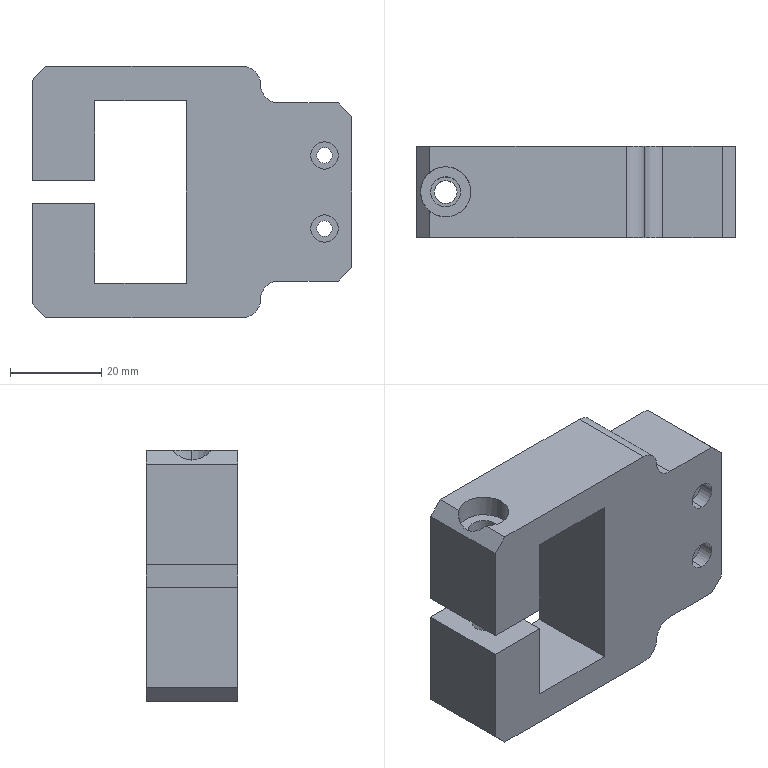Part | SolidWorks | features HoleWzd 3, ICE 3, Chamfer 1, Extrusion 1, Fillet 1 | 1 solid | 41 faces | box 70 x 20 x 55 mm | volume 50750 mm3 | plane 23 | cylinder 18 | commonest cylinder face diameters 3.4 x4 6 x4 8 x4 5 x2 6.6 x2 11 x2
STEP:
#1=CARTESIAN_POINT('',(64.,-6.6,-5.));
#2=VERTEX_POINT('',#1);
#3=CARTESIAN_POINT('',(64.,-6.6,-11.));
#4=VERTEX_POINT('',#3);
#5=CARTESIAN_POINT('',(64.,-6.6,-8.));
#6=DIRECTION('',(0.,-1.,0.));
#7=DIRECTION('',(0.,0.,-1.));
#8=AXIS2_PLACEMENT_3D('',#5,#6,#7);
#9=CIRCLE('',#8,3.);
#10=EDGE_CURVE('',#2,#4,#9,.T.);
#11=ORIENTED_EDGE('',*,*,#10,.F.);
#12=CARTESIAN_POINT('',(64.,-10.,-5.));
#13=VERTEX_POINT('',#12);
#14=CARTESIAN_POINT('',(64.,-10.,-5.));
#15=DIRECTION('',(0.,-1.,0.));
#16=VECTOR('',#15,1000.);
#17=LINE('',#14,#16);
#18=EDGE_CURVE('',#2,#13,#17,.T.);
#19=ORIENTED_EDGE('',*,*,#18,.T.);
#20=CARTESIAN_POINT('',(64.,-10.,-11.));
#21=VERTEX_POINT('',#20);
#22=CARTESIAN_POINT('',(64.,-10.,-8.));
#23=DIRECTION('',(0.,-1.,0.));
#24=DIRECTION('',(0.,0.,-1.));
#25=AXIS2_PLACEMENT_3D('',#22,#23,#24);
#26=CIRCLE('',#25,3.);
#27=EDGE_CURVE('',#13,#21,#26,.T.);
#28=ORIENTED_EDGE('',*,*,#27,.T.);
#29=CARTESIAN_POINT('',(64.,-10.,-11.));
#30=DIRECTION('',(0.,-1.,0.));
#31=VECTOR('',#30,1000.);
#32=LINE('',#29,#31);
#33=EDGE_CURVE('',#4,#21,#32,.T.);
#34=ORIENTED_EDGE('',*,*,#33,.F.);
#35=EDGE_LOOP('',(#11,#19,#28,#34));
#36=FACE_OUTER_BOUND('',#35,.T.);
#37=CARTESIAN_POINT('',(64.,-10.,-8.));
#38=DIRECTION('',(0.,-1.,0.));
#39=DIRECTION('',(0.,0.,-1.));
#40=AXIS2_PLACEMENT_3D('',#37,#38,#39);
#41=CYLINDRICAL_SURFACE('',#40,3.);
#42=ADVANCED_FACE('',(#36),#41,.F.);
#43=CARTESIAN_POINT('',(64.,10.,-6.3));
#44=VERTEX_POINT('',#43);
#45=CARTESIAN_POINT('',(64.,10.,-9.7));
#46=VERTEX_POINT('',#45);
#47=CARTESIAN_POINT('',(64.,10.,-8.));
#48=DIRECTION('',(0.,-1.,0.));
#49=DIRECTION('',(0.,0.,-1.));
#50=AXIS2_PLACEMENT_3D('',#47,#48,#49);
#51=CIRCLE('',#50,1.7);
#52=EDGE_CURVE('',#44,#46,#51,.T.);
#53=ORIENTED_EDGE('',*,*,#52,.F.);
#54=CARTESIAN_POINT('',(64.,-6.6,-6.3));
#55=VERTEX_POINT('',#54);
#56=CARTESIAN_POINT('',(64.,-10.,-6.3));
#57=DIRECTION('',(0.,-1.,0.));
#58=VECTOR('',#57,1000.);
#59=LINE('',#56,#58);
#60=EDGE_CURVE('',#44,#55,#59,.T.);
#61=ORIENTED_EDGE('',*,*,#60,.T.);
#62=CARTESIAN_POINT('',(64.,-6.6,-9.7));
#63=VERTEX_POINT('',#62);
#64=CARTESIAN_POINT('',(64.,-6.6,-8.));
#65=DIRECTION('',(0.,-1.,0.));
#66=DIRECTION('',(0.,0.,-1.));
#67=AXIS2_PLACEMENT_3D('',#64,#65,#66);
#68=CIRCLE('',#67,1.7);
#69=EDGE_CURVE('',#55,#63,#68,.T.);
#70=ORIENTED_EDGE('',*,*,#69,.T.);
#71=CARTESIAN_POINT('',(64.,-10.,-9.7));
#72=DIRECTION('',(0.,-1.,0.));
#73=VECTOR('',#72,1000.);
#74=LINE('',#71,#73);
#75=EDGE_CURVE('',#46,#63,#74,.T.);
#76=ORIENTED_EDGE('',*,*,#75,.F.);
#77=EDGE_LOOP('',(#53,#61,#70,#76));
#78=FACE_OUTER_BOUND('',#77,.T.);
#79=CARTESIAN_POINT('',(64.,-10.,-8.));
#80=DIRECTION('',(0.,-1.,0.));
#81=DIRECTION('',(0.,0.,-1.));
#82=AXIS2_PLACEMENT_3D('',#79,#80,#81);
#83=CYLINDRICAL_SURFACE('',#82,1.7);
#84=ADVANCED_FACE('',(#78),#83,.F.);
#85=CARTESIAN_POINT('',(64.,-6.6,11.));
#86=VERTEX_POINT('',#85);
#87=CARTESIAN_POINT('',(64.,-6.6,5.));
#88=VERTEX_POINT('',#87);
#89=CARTESIAN_POINT('',(64.,-6.6,8.));
#90=DIRECTION('',(0.,-1.,0.));
#91=DIRECTION('',(0.,0.,-1.));
#92=AXIS2_PLACEMENT_3D('',#89,#90,#91);
#93=CIRCLE('',#92,3.);
#94=EDGE_CURVE('',#86,#88,#93,.T.);
#95=ORIENTED_EDGE('',*,*,#94,.F.);
#96=CARTESIAN_POINT('',(64.,-10.,11.));
#97=VERTEX_POINT('',#96);
#98=CARTESIAN_POINT('',(64.,-10.,11.));
#99=DIRECTION('',(0.,-1.,0.));
#100=VECTOR('',#99,1000.);
#101=LINE('',#98,#100);
#102=EDGE_CURVE('',#86,#97,#101,.T.);
#103=ORIENTED_EDGE('',*,*,#102,.T.);
#104=CARTESIAN_POINT('',(64.,-10.,5.));
#105=VERTEX_POINT('',#104);
#106=CARTESIAN_POINT('',(64.,-10.,8.));
#107=DIRECTION('',(0.,-1.,0.));
#108=DIRECTION('',(0.,0.,-1.));
#109=AXIS2_PLACEMENT_3D('',#106,#107,#108);
#110=CIRCLE('',#109,3.);
#111=EDGE_CURVE('',#97,#105,#110,.T.);
#112=ORIENTED_EDGE('',*,*,#111,.T.);
#113=CARTESIAN_POINT('',(64.,-10.,5.));
#114=DIRECTION('',(0.,-1.,0.));
#115=VECTOR('',#114,1000.);
#116=LINE('',#113,#115);
#117=EDGE_CURVE('',#88,#105,#116,.T.);
#118=ORIENTED_EDGE('',*,*,#117,.F.);
#119=EDGE_LOOP('',(#95,#103,#112,#118));
#120=FACE_OUTER_BOUND('',#119,.T.);
#121=CARTESIAN_POINT('',(64.,-10.,8.));
#122=DIRECTION('',(0.,-1.,0.));
#123=DIRECTION('',(0.,0.,-1.));
#124=AXIS2_PLACEMENT_3D('',#121,#122,#123);
#125=CYLINDRICAL_SURFACE('',#124,3.);
#126=ADVANCED_FACE('',(#120),#125,.F.);
#127=CARTESIAN_POINT('',(64.,10.,9.7));
#128=VERTEX_POINT('',#127);
#129=CARTESIAN_POINT('',(64.,10.,6.3));
#130=VERTEX_POINT('',#129);
#131=CARTESIAN_POINT('',(64.,10.,8.));
#132=DIRECTION('',(0.,-1.,0.));
#133=DIRECTION('',(0.,0.,-1.));
#134=AXIS2_PLACEMENT_3D('',#131,#132,#133);
#135=CIRCLE('',#134,1.7);
#136=EDGE_CURVE('',#128,#130,#135,.T.);
#137=ORIENTED_EDGE('',*,*,#136,.F.);
#138=CARTESIAN_POINT('',(64.,-6.6,9.7));
#139=VERTEX_POINT('',#138);
#140=CARTESIAN_POINT('',(64.,-10.,9.7));
#141=DIRECTION('',(0.,-1.,0.));
#142=VECTOR('',#141,1000.);
#143=LINE('',#140,#142);
#144=EDGE_CURVE('',#128,#139,#143,.T.);
#145=ORIENTED_EDGE('',*,*,#144,.T.);
#146=CARTESIAN_POINT('',(64.,-6.6,6.3));
#147=VERTEX_POINT('',#146);
#148=CARTESIAN_POINT('',(64.,-6.6,8.));
#149=DIRECTION('',(0.,-1.,0.));
#150=DIRECTION('',(0.,0.,-1.));
#151=AXIS2_PLACEMENT_3D('',#148,#149,#150);
#152=CIRCLE('',#151,1.7);
#153=EDGE_CURVE('',#139,#147,#152,.T.);
#154=ORIENTED_EDGE('',*,*,#153,.T.);
#155=CARTESIAN_POINT('',(64.,-10.,6.3));
#156=DIRECTION('',(0.,-1.,0.));
#157=VECTOR('',#156,1000.);
#158=LINE('',#155,#157);
#159=EDGE_CURVE('',#130,#147,#158,.T.);
#160=ORIENTED_EDGE('',*,*,#159,.F.);
#161=EDGE_LOOP('',(#137,#145,#154,#160));
#162=FACE_OUTER_BOUND('',#161,.T.);
#163=CARTESIAN_POINT('',(64.,-10.,8.));
#164=DIRECTION('',(0.,-1.,0.));
#165=DIRECTION('',(0.,0.,-1.));
#166=AXIS2_PLACEMENT_3D('',#163,#164,#165);
#167=CYLINDRICAL_SURFACE('',#166,1.7);
#168=ADVANCED_FACE('',(#162),#167,.F.);
#169=CARTESIAN_POINT('',(3.969,0.,-27.5));
#170=VERTEX_POINT('',#169);
#171=CARTESIAN_POINT('',(8.969,0.,-27.5));
#172=VERTEX_POINT('',#171);
#173=CARTESIAN_POINT('',(6.469,0.,-27.5));
#174=DIRECTION('',(0.,0.,1.));
#175=DIRECTION('',(1.,0.,0.));
#176=AXIS2_PLACEMENT_3D('',#173,#174,#175);
#177=CIRCLE('',#176,2.5);
#178=EDGE_CURVE('',#170,#172,#177,.T.);
#179=ORIENTED_EDGE('',*,*,#178,.F.);
#180=CARTESIAN_POINT('',(3.969,0.,-2.5));
#181=VERTEX_POINT('',#180);
#182=CARTESIAN_POINT('',(3.969,0.,-2.5));
#183=DIRECTION('',(0.,0.,1.));
#184=VECTOR('',#183,1000.);
#185=LINE('',#182,#184);
#186=EDGE_CURVE('',#170,#181,#185,.T.);
#187=ORIENTED_EDGE('',*,*,#186,.T.);
#188=CARTESIAN_POINT('',(8.969,0.,-2.5));
#189=VERTEX_POINT('',#188);
#190=CARTESIAN_POINT('',(6.469,0.,-2.5));
#191=DIRECTION('',(0.,0.,1.));
#192=DIRECTION('',(1.,0.,0.));
#193=AXIS2_PLACEMENT_3D('',#190,#191,#192);
#194=CIRCLE('',#193,2.5);
#195=EDGE_CURVE('',#181,#189,#194,.T.);
#196=ORIENTED_EDGE('',*,*,#195,.T.);
#197=CARTESIAN_POINT('',(8.969,0.,-2.5));
#198=DIRECTION('',(0.,0.,1.));
#199=VECTOR('',#198,1000.);
#200=LINE('',#197,#199);
#201=EDGE_CURVE('',#172,#189,#200,.T.);
#202=ORIENTED_EDGE('',*,*,#201,.F.);
#203=EDGE_LOOP('',(#179,#187,#196,#202));
#204=FACE_OUTER_BOUND('',#203,.T.);
#205=CARTESIAN_POINT('',(6.469,0.,-2.5));
#206=DIRECTION('',(0.,0.,1.));
#207=DIRECTION('',(1.,0.,0.));
#208=AXIS2_PLACEMENT_3D('',#205,#206,#207);
#209=CYLINDRICAL_SURFACE('',#208,2.5);
#210=ADVANCED_FACE('',(#204),#209,.F.);
#211=CARTESIAN_POINT('',(0.969,0.,22.8));
#212=VERTEX_POINT('',#211);
#213=CARTESIAN_POINT('',(11.969,0.,22.8));
#214=VERTEX_POINT('',#213);
#215=CARTESIAN_POINT('',(6.469,0.,22.8));
#216=DIRECTION('',(0.,0.,1.));
#217=DIRECTION('',(1.,0.,0.));
#218=AXIS2_PLACEMENT_3D('',#215,#216,#217);
#219=CIRCLE('',#218,5.5);
#220=EDGE_CURVE('',#212,#214,#219,.T.);
#221=ORIENTED_EDGE('',*,*,#220,.F.);
#222=CARTESIAN_POINT('',(0.969,0.,25.469));
#223=VERTEX_POINT('',#222);
#224=CARTESIAN_POINT('',(0.969,0.,27.5));
#225=DIRECTION('',(0.,0.,1.));
#226=VECTOR('',#225,1000.);
#227=LINE('',#224,#226);
#228=EDGE_CURVE('',#212,#223,#227,.T.);
#229=ORIENTED_EDGE('',*,*,#228,.T.);
#230=CARTESIAN_POINT('',(3.,-4.268,27.5));
#231=VERTEX_POINT('',#230);
#232=CARTESIAN_POINT('',(0.969,0.,25.469));
#233=CARTESIAN_POINT('',(0.969,-1.685,25.469));
#234=CARTESIAN_POINT('',(1.693,-3.206,26.193));
#235=CARTESIAN_POINT('',(3.,-4.268,27.5));
#236=(BOUNDED_CURVE()B_SPLINE_CURVE(3,(#232,#233,#234,#235),.UNSPECIFIED.,.F.,.F.)B_SPLINE_CURVE_WITH_KNOTS((4,4),(3.142,4.03),.UNSPECIFIED.)CURVE()GEOMETRIC_REPRESENTATION_ITEM()RATIONAL_B_SPLINE_CURVE((1.,0.9353,0.9353,1.))REPRESENTATION_ITEM(''));
#237=EDGE_CURVE('',#223,#231,#236,.T.);
#238=ORIENTED_EDGE('',*,*,#237,.T.);
#239=CARTESIAN_POINT('',(11.969,0.,27.5));
#240=VERTEX_POINT('',#239);
#241=CARTESIAN_POINT('',(6.469,0.,27.5));
#242=DIRECTION('',(0.,0.,1.));
#243=DIRECTION('',(1.,0.,0.));
#244=AXIS2_PLACEMENT_3D('',#241,#242,#243);
#245=CIRCLE('',#244,5.5);
#246=EDGE_CURVE('',#231,#240,#245,.T.);
#247=ORIENTED_EDGE('',*,*,#246,.T.);
#248=CARTESIAN_POINT('',(11.969,0.,27.5));
#249=DIRECTION('',(0.,0.,1.));
#250=VECTOR('',#249,1000.);
#251=LINE('',#248,#250);
#252=EDGE_CURVE('',#214,#240,#251,.T.);
#253=ORIENTED_EDGE('',*,*,#252,.F.);
#254=EDGE_LOOP('',(#221,#229,#238,#247,#253));
#255=FACE_OUTER_BOUND('',#254,.T.);
#256=CARTESIAN_POINT('',(6.469,0.,27.5));
#257=DIRECTION('',(0.,0.,1.));
#258=DIRECTION('',(1.,0.,0.));
#259=AXIS2_PLACEMENT_3D('',#256,#257,#258);
#260=CYLINDRICAL_SURFACE('',#259,5.5);
#261=ADVANCED_FACE('',(#255),#260,.F.);
#262=CARTESIAN_POINT('',(9.769,0.,2.5));
#263=VERTEX_POINT('',#262);
#264=CARTESIAN_POINT('',(3.169,0.,2.5));
#265=VERTEX_POINT('',#264);
#266=CARTESIAN_POINT('',(6.469,0.,2.5));
#267=DIRECTION('',(0.,0.,-1.));
#268=DIRECTION('',(1.,0.,0.));
#269=AXIS2_PLACEMENT_3D('',#266,#267,#268);
#270=CIRCLE('',#269,3.3);
#271=EDGE_CURVE('',#263,#265,#270,.T.);
#272=ORIENTED_EDGE('',*,*,#271,.T.);
#273=CARTESIAN_POINT('',(3.169,0.,22.8));
#274=VERTEX_POINT('',#273);
#275=CARTESIAN_POINT('',(3.169,0.,27.5));
#276=DIRECTION('',(0.,0.,1.));
#277=VECTOR('',#276,1000.);
#278=LINE('',#275,#277);
#279=EDGE_CURVE('',#265,#274,#278,.T.);
#280=ORIENTED_EDGE('',*,*,#279,.T.);
#281=CARTESIAN_POINT('',(9.769,0.,22.8));
#282=VERTEX_POINT('',#281);
#283=CARTESIAN_POINT('',(6.469,0.,22.8));
#284=DIRECTION('',(0.,0.,1.));
#285=DIRECTION('',(1.,0.,0.));
#286=AXIS2_PLACEMENT_3D('',#283,#284,#285);
#287=CIRCLE('',#286,3.3);
#288=EDGE_CURVE('',#274,#282,#287,.T.);
#289=ORIENTED_EDGE('',*,*,#288,.T.);
#290=CARTESIAN_POINT('',(9.769,0.,27.5));
#291=DIRECTION('',(0.,0.,1.));
#292=VECTOR('',#291,1000.);
#293=LINE('',#290,#292);
#294=EDGE_CURVE('',#263,#282,#293,.T.);
#295=ORIENTED_EDGE('',*,*,#294,.F.);
#296=EDGE_LOOP('',(#272,#280,#289,#295));
#297=FACE_OUTER_BOUND('',#296,.T.);
#298=CARTESIAN_POINT('',(6.469,0.,27.5));
#299=DIRECTION('',(0.,0.,1.));
#300=DIRECTION('',(1.,0.,0.));
#301=AXIS2_PLACEMENT_3D('',#298,#299,#300);
#302=CYLINDRICAL_SURFACE('',#301,3.3);
#303=ADVANCED_FACE('',(#297),#302,.F.);
#304=CARTESIAN_POINT('',(0.,-10.,24.5));
#305=VERTEX_POINT('',#304);
#306=CARTESIAN_POINT('',(0.,-10.,2.5));
#307=VERTEX_POINT('',#306);
#308=CARTESIAN_POINT('',(0.,-10.,27.5));
#309=DIRECTION('',(0.,0.,-1.));
#310=VECTOR('',#309,1000.);
#311=LINE('',#308,#310);
#312=EDGE_CURVE('',#305,#307,#311,.T.);
#313=ORIENTED_EDGE('',*,*,#312,.F.);
#314=CARTESIAN_POINT('',(0.,10.,24.5));
#315=VERTEX_POINT('',#314);
#316=CARTESIAN_POINT('',(0.,0.,24.5));
#317=DIRECTION('',(0.,1.,0.));
#318=VECTOR('',#317,1000.);
#319=LINE('',#316,#318);
#320=EDGE_CURVE('',#305,#315,#319,.T.);
#321=ORIENTED_EDGE('',*,*,#320,.T.);
#322=CARTESIAN_POINT('',(0.,10.,2.5));
#323=VERTEX_POINT('',#322);
#324=CARTESIAN_POINT('',(0.,10.,27.5));
#325=DIRECTION('',(0.,0.,1.));
#326=VECTOR('',#325,1000.);
#327=LINE('',#324,#326);
#328=EDGE_CURVE('',#323,#315,#327,.T.);
#329=ORIENTED_EDGE('',*,*,#328,.F.);
#330=CARTESIAN_POINT('',(0.,10.,2.5));
#331=DIRECTION('',(0.,-1.,0.));
#332=VECTOR('',#331,1000.);
#333=LINE('',#330,#332);
#334=EDGE_CURVE('',#323,#307,#333,.T.);
#335=ORIENTED_EDGE('',*,*,#334,.T.);
#336=EDGE_LOOP('',(#313,#321,#329,#335));
#337=FACE_OUTER_BOUND('',#336,.T.);
#338=CARTESIAN_POINT('',(0.,0.,0.));
#339=DIRECTION('',(1.,0.,0.));
#340=DIRECTION('',(0.,0.,-1.));
#341=AXIS2_PLACEMENT_3D('',#338,#339,#340);
#342=PLANE('',#341);
#343=ADVANCED_FACE('',(#337),#342,.F.);
#344=CARTESIAN_POINT('',(13.743,-10.,20.));
#345=VERTEX_POINT('',#344);
#346=CARTESIAN_POINT('',(13.743,-10.,2.5));
#347=VERTEX_POINT('',#346);
#348=CARTESIAN_POINT('',(13.743,-10.,20.));
#349=DIRECTION('',(0.,0.,-1.));
#350=VECTOR('',#349,1000.);
#351=LINE('',#348,#350);
#352=EDGE_CURVE('',#345,#347,#351,.T.);
#353=ORIENTED_EDGE('',*,*,#352,.T.);
#354=CARTESIAN_POINT('',(13.743,10.,2.5));
#355=VERTEX_POINT('',#354);
#356=CARTESIAN_POINT('',(13.743,10.,2.5));
#357=DIRECTION('',(0.,-1.,0.));
#358=VECTOR('',#357,1000.);
#359=LINE('',#356,#358);
#360=EDGE_CURVE('',#355,#347,#359,.T.);
#361=ORIENTED_EDGE('',*,*,#360,.F.);
#362=CARTESIAN_POINT('',(13.743,10.,20.));
#363=VERTEX_POINT('',#362);
#364=CARTESIAN_POINT('',(13.743,10.,20.));
#365=DIRECTION('',(0.,0.,-1.));
#366=VECTOR('',#365,1000.);
#367=LINE('',#364,#366);
#368=EDGE_CURVE('',#363,#355,#367,.T.);
#369=ORIENTED_EDGE('',*,*,#368,.F.);
#370=CARTESIAN_POINT('',(13.743,10.,20.));
#371=DIRECTION('',(0.,-1.,0.));
#372=VECTOR('',#371,1000.);
#373=LINE('',#370,#372);
#374=EDGE_CURVE('',#363,#345,#373,.T.);
#375=ORIENTED_EDGE('',*,*,#374,.T.);
#376=EDGE_LOOP('',(#353,#361,#369,#375));
#377=FACE_OUTER_BOUND('',#376,.T.);
#378=CARTESIAN_POINT('',(13.743,10.,20.));
#379=DIRECTION('',(-1.,0.,0.));
#380=DIRECTION('',(0.,0.,1.));
#381=AXIS2_PLACEMENT_3D('',#378,#379,#380);
#382=PLANE('',#381);
#383=ADVANCED_FACE('',(#377),#382,.F.);
#384=CARTESIAN_POINT('',(6.469,0.,-27.5));
#385=DIRECTION('',(0.,0.,1.));
#386=DIRECTION('',(1.,0.,0.));
#387=AXIS2_PLACEMENT_3D('',#384,#385,#386);
#388=CIRCLE('',#387,2.5);
#389=EDGE_CURVE('',#172,#170,#388,.T.);
#390=ORIENTED_EDGE('',*,*,#389,.T.);
#391=ORIENTED_EDGE('',*,*,#178,.T.);
#392=EDGE_LOOP('',(#390,#391));
#393=FACE_BOUND('',#392,.T.);
#394=CARTESIAN_POINT('',(46.,-10.,-27.5));
#395=VERTEX_POINT('',#394);
#396=CARTESIAN_POINT('',(3.,-10.,-27.5));
#397=VERTEX_POINT('',#396);
#398=CARTESIAN_POINT('',(70.,-10.,-27.5));
#399=DIRECTION('',(-1.,0.,0.));
#400=VECTOR('',#399,1000.);
#401=LINE('',#398,#400);
#402=EDGE_CURVE('',#395,#397,#401,.T.);
#403=ORIENTED_EDGE('',*,*,#402,.T.);
#404=CARTESIAN_POINT('',(3.,10.,-27.5));
#405=VERTEX_POINT('',#404);
#406=CARTESIAN_POINT('',(3.,10.,-27.5));
#407=DIRECTION('',(0.,1.,0.));
#408=VECTOR('',#407,1000.);
#409=LINE('',#406,#408);
#410=EDGE_CURVE('',#397,#405,#409,.T.);
#411=ORIENTED_EDGE('',*,*,#410,.T.);
#412=CARTESIAN_POINT('',(46.,10.,-27.5));
#413=VERTEX_POINT('',#412);
#414=CARTESIAN_POINT('',(70.,10.,-27.5));
#415=DIRECTION('',(-1.,0.,0.));
#416=VECTOR('',#415,1000.);
#417=LINE('',#414,#416);
#418=EDGE_CURVE('',#413,#405,#417,.T.);
#419=ORIENTED_EDGE('',*,*,#418,.F.);
#420=CARTESIAN_POINT('',(46.,10.,-27.5));
#421=DIRECTION('',(0.,-1.,0.));
#422=VECTOR('',#421,1000.);
#423=LINE('',#420,#422);
#424=EDGE_CURVE('',#413,#395,#423,.T.);
#425=ORIENTED_EDGE('',*,*,#424,.T.);
#426=EDGE_LOOP('',(#403,#411,#419,#425));
#427=FACE_OUTER_BOUND('',#426,.T.);
#428=CARTESIAN_POINT('',(70.,10.,-27.5));
#429=DIRECTION('',(0.,0.,1.));
#430=DIRECTION('',(0.,-1.,0.));
#431=AXIS2_PLACEMENT_3D('',#428,#429,#430);
#432=PLANE('',#431);
#433=ADVANCED_FACE('',(#393,#427),#432,.F.);
#434=CARTESIAN_POINT('',(64.,10.,-8.));
#435=DIRECTION('',(0.,-1.,0.));
#436=DIRECTION('',(0.,0.,-1.));
#437=AXIS2_PLACEMENT_3D('',#434,#435,#436);
#438=CIRCLE('',#437,1.7);
#439=EDGE_CURVE('',#46,#44,#438,.T.);
#440=ORIENTED_EDGE('',*,*,#439,.T.);
#441=ORIENTED_EDGE('',*,*,#52,.T.);
#442=EDGE_LOOP('',(#440,#441));
#443=FACE_BOUND('',#442,.T.);
#444=CARTESIAN_POINT('',(64.,10.,8.));
#445=DIRECTION('',(0.,-1.,0.));
#446=DIRECTION('',(0.,0.,-1.));
#447=AXIS2_PLACEMENT_3D('',#444,#445,#446);
#448=CIRCLE('',#447,1.7);
#449=EDGE_CURVE('',#130,#128,#448,.T.);
#450=ORIENTED_EDGE('',*,*,#449,.T.);
#451=ORIENTED_EDGE('',*,*,#136,.T.);
#452=EDGE_LOOP('',(#450,#451));
#453=FACE_BOUND('',#452,.T.);
#454=ORIENTED_EDGE('',*,*,#328,.T.);
#455=CARTESIAN_POINT('',(3.,10.,27.5));
#456=VERTEX_POINT('',#455);
#457=CARTESIAN_POINT('',(3.,10.,27.5));
#458=DIRECTION('',(0.7071,0.,0.7071));
#459=VECTOR('',#458,1000.);
#460=LINE('',#457,#459);
#461=EDGE_CURVE('',#315,#456,#460,.T.);
#462=ORIENTED_EDGE('',*,*,#461,.T.);
#463=CARTESIAN_POINT('',(46.,10.,27.5));
#464=VERTEX_POINT('',#463);
#465=CARTESIAN_POINT('',(70.,10.,27.5));
#466=DIRECTION('',(-1.,0.,0.));
#467=VECTOR('',#466,1000.);
#468=LINE('',#465,#467);
#469=EDGE_CURVE('',#464,#456,#468,.T.);
#470=ORIENTED_EDGE('',*,*,#469,.F.);
#471=CARTESIAN_POINT('',(50.,10.,23.5));
#472=VERTEX_POINT('',#471);
#473=CARTESIAN_POINT('',(46.,10.,23.5));
#474=DIRECTION('',(0.,1.,0.));
#475=DIRECTION('',(0.,0.,-1.));
#476=AXIS2_PLACEMENT_3D('',#473,#474,#475);
#477=CIRCLE('',#476,4.);
#478=EDGE_CURVE('',#464,#472,#477,.T.);
#479=ORIENTED_EDGE('',*,*,#478,.T.);
#480=CARTESIAN_POINT('',(54.,10.,19.5));
#481=VERTEX_POINT('',#480);
#482=CARTESIAN_POINT('',(54.,10.,23.5));
#483=DIRECTION('',(0.,-1.,0.));
#484=DIRECTION('',(0.,0.,-1.));
#485=AXIS2_PLACEMENT_3D('',#482,#483,#484);
#486=CIRCLE('',#485,4.);
#487=EDGE_CURVE('',#472,#481,#486,.T.);
#488=ORIENTED_EDGE('',*,*,#487,.T.);
#489=CARTESIAN_POINT('',(67.,10.,19.5));
#490=VERTEX_POINT('',#489);
#491=CARTESIAN_POINT('',(70.,10.,19.5));
#492=DIRECTION('',(-1.,0.,0.));
#493=VECTOR('',#492,1000.);
#494=LINE('',#491,#493);
#495=EDGE_CURVE('',#490,#481,#494,.T.);
#496=ORIENTED_EDGE('',*,*,#495,.F.);
#497=CARTESIAN_POINT('',(70.,10.,16.5));
#498=VERTEX_POINT('',#497);
#499=CARTESIAN_POINT('',(67.,10.,19.5));
#500=DIRECTION('',(0.7071,0.,-0.7071));
#501=VECTOR('',#500,1000.);
#502=LINE('',#499,#501);
#503=EDGE_CURVE('',#490,#498,#502,.T.);
#504=ORIENTED_EDGE('',*,*,#503,.T.);
#505=CARTESIAN_POINT('',(70.,10.,-16.5));
#506=VERTEX_POINT('',#505);
#507=CARTESIAN_POINT('',(70.,10.,27.5));
#508=DIRECTION('',(0.,0.,1.));
#509=VECTOR('',#508,1000.);
#510=LINE('',#507,#509);
#511=EDGE_CURVE('',#506,#498,#510,.T.);
#512=ORIENTED_EDGE('',*,*,#511,.F.);
#513=CARTESIAN_POINT('',(67.,10.,-19.5));
#514=VERTEX_POINT('',#513);
#515=CARTESIAN_POINT('',(70.,10.,-16.5));
#516=DIRECTION('',(-0.7071,0.,-0.7071));
#517=VECTOR('',#516,1000.);
#518=LINE('',#515,#517);
#519=EDGE_CURVE('',#506,#514,#518,.T.);
#520=ORIENTED_EDGE('',*,*,#519,.T.);
#521=CARTESIAN_POINT('',(54.,10.,-19.5));
#522=VERTEX_POINT('',#521);
#523=CARTESIAN_POINT('',(70.,10.,-19.5));
#524=DIRECTION('',(1.,0.,0.));
#525=VECTOR('',#524,1000.);
#526=LINE('',#523,#525);
#527=EDGE_CURVE('',#522,#514,#526,.T.);
#528=ORIENTED_EDGE('',*,*,#527,.F.);
#529=CARTESIAN_POINT('',(50.,10.,-23.5));
#530=VERTEX_POINT('',#529);
#531=CARTESIAN_POINT('',(54.,10.,-23.5));
#532=DIRECTION('',(0.,-1.,0.));
#533=DIRECTION('',(0.,0.,-1.));
#534=AXIS2_PLACEMENT_3D('',#531,#532,#533);
#535=CIRCLE('',#534,4.);
#536=EDGE_CURVE('',#522,#530,#535,.T.);
#537=ORIENTED_EDGE('',*,*,#536,.T.);
#538=CARTESIAN_POINT('',(46.,10.,-23.5));
#539=DIRECTION('',(0.,1.,0.));
#540=DIRECTION('',(0.,0.,-1.));
#541=AXIS2_PLACEMENT_3D('',#538,#539,#540);
#542=CIRCLE('',#541,4.);
#543=EDGE_CURVE('',#530,#413,#542,.T.);
#544=ORIENTED_EDGE('',*,*,#543,.T.);
#545=ORIENTED_EDGE('',*,*,#418,.T.);
#546=CARTESIAN_POINT('',(0.,10.,-24.5));
#547=VERTEX_POINT('',#546);
#548=CARTESIAN_POINT('',(3.,10.,-27.5));
#549=DIRECTION('',(-0.7071,0.,0.7071));
#550=VECTOR('',#549,1000.);
#551=LINE('',#548,#550);
#552=EDGE_CURVE('',#405,#547,#551,.T.);
#553=ORIENTED_EDGE('',*,*,#552,.T.);
#554=CARTESIAN_POINT('',(0.,10.,-2.5));
#555=VERTEX_POINT('',#554);
#556=CARTESIAN_POINT('',(0.,10.,27.5));
#557=DIRECTION('',(0.,0.,1.));
#558=VECTOR('',#557,1000.);
#559=LINE('',#556,#558);
#560=EDGE_CURVE('',#547,#555,#559,.T.);
#561=ORIENTED_EDGE('',*,*,#560,.T.);
#562=CARTESIAN_POINT('',(13.743,10.,-2.5));
#563=VERTEX_POINT('',#562);
#564=CARTESIAN_POINT('',(0.,10.,-2.5));
#565=DIRECTION('',(1.,0.,0.));
#566=VECTOR('',#565,1000.);
#567=LINE('',#564,#566);
#568=EDGE_CURVE('',#555,#563,#567,.T.);
#569=ORIENTED_EDGE('',*,*,#568,.T.);
#570=CARTESIAN_POINT('',(13.743,10.,-20.));
#571=VERTEX_POINT('',#570);
#572=CARTESIAN_POINT('',(13.743,10.,20.));
#573=DIRECTION('',(0.,0.,-1.));
#574=VECTOR('',#573,1000.);
#575=LINE('',#572,#574);
#576=EDGE_CURVE('',#563,#571,#575,.T.);
#577=ORIENTED_EDGE('',*,*,#576,.T.);
#578=CARTESIAN_POINT('',(33.743,10.,-20.));
#579=VERTEX_POINT('',#578);
#580=CARTESIAN_POINT('',(13.743,10.,-20.));
#581=DIRECTION('',(1.,0.,0.));
#582=VECTOR('',#581,1000.);
#583=LINE('',#580,#582);
#584=EDGE_CURVE('',#571,#579,#583,.T.);
#585=ORIENTED_EDGE('',*,*,#584,.T.);
#586=CARTESIAN_POINT('',(33.743,10.,20.));
#587=VERTEX_POINT('',#586);
#588=CARTESIAN_POINT('',(33.743,10.,20.));
#589=DIRECTION('',(0.,0.,1.));
#590=VECTOR('',#589,1000.);
#591=LINE('',#588,#590);
#592=EDGE_CURVE('',#579,#587,#591,.T.);
#593=ORIENTED_EDGE('',*,*,#592,.T.);
#594=CARTESIAN_POINT('',(13.743,10.,20.));
#595=DIRECTION('',(-1.,0.,0.));
#596=VECTOR('',#595,1000.);
#597=LINE('',#594,#596);
#598=EDGE_CURVE('',#587,#363,#597,.T.);
#599=ORIENTED_EDGE('',*,*,#598,.T.);
#600=ORIENTED_EDGE('',*,*,#368,.T.);
#601=CARTESIAN_POINT('',(0.,10.,2.5));
#602=DIRECTION('',(-1.,0.,0.));
#603=VECTOR('',#602,1000.);
#604=LINE('',#601,#603);
#605=EDGE_CURVE('',#355,#323,#604,.T.);
#606=ORIENTED_EDGE('',*,*,#605,.T.);
#607=EDGE_LOOP('',(#454,#462,#470,#479,#488,#496,#504,#512,#520,#528,#537,#544,#545,#553,#561,#569,#577,#585,#593,#599,#600,#606));
#608=FACE_OUTER_BOUND('',#607,.T.);
#609=CARTESIAN_POINT('',(70.,10.,27.5));
#610=DIRECTION('',(0.,-1.,0.));
#611=DIRECTION('',(0.,0.,-1.));
#612=AXIS2_PLACEMENT_3D('',#609,#610,#611);
#613=PLANE('',#612);
#614=ADVANCED_FACE('',(#443,#453,#608),#613,.F.);
#615=ORIENTED_EDGE('',*,*,#469,.T.);
#616=CARTESIAN_POINT('',(3.,4.268,27.5));
#617=VERTEX_POINT('',#616);
#618=CARTESIAN_POINT('',(3.,10.,27.5));
#619=DIRECTION('',(0.,-1.,0.));
#620=VECTOR('',#619,1000.);
#621=LINE('',#618,#620);
#622=EDGE_CURVE('',#456,#617,#621,.T.);
#623=ORIENTED_EDGE('',*,*,#622,.T.);
#624=CARTESIAN_POINT('',(6.469,0.,27.5));
#625=DIRECTION('',(0.,0.,1.));
#626=DIRECTION('',(1.,0.,0.));
#627=AXIS2_PLACEMENT_3D('',#624,#625,#626);
#628=CIRCLE('',#627,5.5);
#629=EDGE_CURVE('',#240,#617,#628,.T.);
#630=ORIENTED_EDGE('',*,*,#629,.F.);
#631=ORIENTED_EDGE('',*,*,#246,.F.);
#632=CARTESIAN_POINT('',(3.,-10.,27.5));
#633=VERTEX_POINT('',#632);
#634=CARTESIAN_POINT('',(3.,10.,27.5));
#635=DIRECTION('',(0.,-1.,0.));
#636=VECTOR('',#635,1000.);
#637=LINE('',#634,#636);
#638=EDGE_CURVE('',#231,#633,#637,.T.);
#639=ORIENTED_EDGE('',*,*,#638,.T.);
#640=CARTESIAN_POINT('',(46.,-10.,27.5));
#641=VERTEX_POINT('',#640);
#642=CARTESIAN_POINT('',(70.,-10.,27.5));
#643=DIRECTION('',(-1.,0.,0.));
#644=VECTOR('',#643,1000.);
#645=LINE('',#642,#644);
#646=EDGE_CURVE('',#641,#633,#645,.T.);
#647=ORIENTED_EDGE('',*,*,#646,.F.);
#648=CARTESIAN_POINT('',(46.,10.,27.5));
#649=DIRECTION('',(0.,1.,0.));
#650=VECTOR('',#649,1000.);
#651=LINE('',#648,#650);
#652=EDGE_CURVE('',#641,#464,#651,.T.);
#653=ORIENTED_EDGE('',*,*,#652,.T.);
#654=EDGE_LOOP('',(#615,#623,#630,#631,#639,#647,#653));
#655=FACE_OUTER_BOUND('',#654,.T.);
#656=CARTESIAN_POINT('',(70.,10.,27.5));
#657=DIRECTION('',(0.,0.,-1.));
#658=DIRECTION('',(-1.,0.,0.));
#659=AXIS2_PLACEMENT_3D('',#656,#657,#658);
#660=PLANE('',#659);
#661=ADVANCED_FACE('',(#655),#660,.F.);
#662=CARTESIAN_POINT('',(64.,-10.,-8.));
#663=DIRECTION('',(0.,-1.,0.));
#664=DIRECTION('',(0.,0.,-1.));
#665=AXIS2_PLACEMENT_3D('',#662,#663,#664);
#666=CIRCLE('',#665,3.);
#667=EDGE_CURVE('',#21,#13,#666,.T.);
#668=ORIENTED_EDGE('',*,*,#667,.F.);
#669=ORIENTED_EDGE('',*,*,#27,.F.);
#670=EDGE_LOOP('',(#668,#669));
#671=FACE_BOUND('',#670,.T.);
#672=CARTESIAN_POINT('',(64.,-10.,8.));
#673=DIRECTION('',(0.,-1.,0.));
#674=DIRECTION('',(0.,0.,-1.));
#675=AXIS2_PLACEMENT_3D('',#672,#673,#674);
#676=CIRCLE('',#675,3.);
#677=EDGE_CURVE('',#105,#97,#676,.T.);
#678=ORIENTED_EDGE('',*,*,#677,.F.);
#679=ORIENTED_EDGE('',*,*,#111,.F.);
#680=EDGE_LOOP('',(#678,#679));
#681=FACE_BOUND('',#680,.T.);
#682=ORIENTED_EDGE('',*,*,#646,.T.);
#683=CARTESIAN_POINT('',(3.,-10.,27.5));
#684=DIRECTION('',(-0.7071,0.,-0.7071));
#685=VECTOR('',#684,1000.);
#686=LINE('',#683,#685);
#687=EDGE_CURVE('',#633,#305,#686,.T.);
#688=ORIENTED_EDGE('',*,*,#687,.T.);
#689=ORIENTED_EDGE('',*,*,#312,.T.);
#690=CARTESIAN_POINT('',(0.,-10.,2.5));
#691=DIRECTION('',(-1.,0.,0.));
#692=VECTOR('',#691,1000.);
#693=LINE('',#690,#692);
#694=EDGE_CURVE('',#347,#307,#693,.T.);
#695=ORIENTED_EDGE('',*,*,#694,.F.);
#696=ORIENTED_EDGE('',*,*,#352,.F.);
#697=CARTESIAN_POINT('',(33.743,-10.,20.));
#698=VERTEX_POINT('',#697);
#699=CARTESIAN_POINT('',(13.743,-10.,20.));
#700=DIRECTION('',(-1.,0.,0.));
#701=VECTOR('',#700,1000.);
#702=LINE('',#699,#701);
#703=EDGE_CURVE('',#698,#345,#702,.T.);
#704=ORIENTED_EDGE('',*,*,#703,.F.);
#705=CARTESIAN_POINT('',(33.743,-10.,-20.));
#706=VERTEX_POINT('',#705);
#707=CARTESIAN_POINT('',(33.743,-10.,20.));
#708=DIRECTION('',(0.,0.,1.));
#709=VECTOR('',#708,1000.);
#710=LINE('',#707,#709);
#711=EDGE_CURVE('',#706,#698,#710,.T.);
#712=ORIENTED_EDGE('',*,*,#711,.F.);
#713=CARTESIAN_POINT('',(13.743,-10.,-20.));
#714=VERTEX_POINT('',#713);
#715=CARTESIAN_POINT('',(13.743,-10.,-20.));
#716=DIRECTION('',(1.,0.,0.));
#717=VECTOR('',#716,1000.);
#718=LINE('',#715,#717);
#719=EDGE_CURVE('',#714,#706,#718,.T.);
#720=ORIENTED_EDGE('',*,*,#719,.F.);
#721=CARTESIAN_POINT('',(13.743,-10.,-2.5));
#722=VERTEX_POINT('',#721);
#723=CARTESIAN_POINT('',(13.743,-10.,20.));
#724=DIRECTION('',(0.,0.,-1.));
#725=VECTOR('',#724,1000.);
#726=LINE('',#723,#725);
#727=EDGE_CURVE('',#722,#714,#726,.T.);
#728=ORIENTED_EDGE('',*,*,#727,.F.);
#729=CARTESIAN_POINT('',(0.,-10.,-2.5));
#730=VERTEX_POINT('',#729);
#731=CARTESIAN_POINT('',(0.,-10.,-2.5));
#732=DIRECTION('',(1.,0.,0.));
#733=VECTOR('',#732,1000.);
#734=LINE('',#731,#733);
#735=EDGE_CURVE('',#730,#722,#734,.T.);
#736=ORIENTED_EDGE('',*,*,#735,.F.);
#737=CARTESIAN_POINT('',(0.,-10.,-24.5));
#738=VERTEX_POINT('',#737);
#739=CARTESIAN_POINT('',(0.,-10.,27.5));
#740=DIRECTION('',(0.,0.,-1.));
#741=VECTOR('',#740,1000.);
#742=LINE('',#739,#741);
#743=EDGE_CURVE('',#730,#738,#742,.T.);
#744=ORIENTED_EDGE('',*,*,#743,.T.);
#745=CARTESIAN_POINT('',(3.,-10.,-27.5));
#746=DIRECTION('',(0.7071,0.,-0.7071));
#747=VECTOR('',#746,1000.);
#748=LINE('',#745,#747);
#749=EDGE_CURVE('',#738,#397,#748,.T.);
#750=ORIENTED_EDGE('',*,*,#749,.T.);
#751=ORIENTED_EDGE('',*,*,#402,.F.);
#752=CARTESIAN_POINT('',(50.,-10.,-23.5));
#753=VERTEX_POINT('',#752);
#754=CARTESIAN_POINT('',(46.,-10.,-23.5));
#755=DIRECTION('',(0.,-1.,0.));
#756=DIRECTION('',(0.,0.,1.));
#757=AXIS2_PLACEMENT_3D('',#754,#755,#756);
#758=CIRCLE('',#757,4.);
#759=EDGE_CURVE('',#395,#753,#758,.T.);
#760=ORIENTED_EDGE('',*,*,#759,.T.);
#761=CARTESIAN_POINT('',(54.,-10.,-19.5));
#762=VERTEX_POINT('',#761);
#763=CARTESIAN_POINT('',(54.,-10.,-23.5));
#764=DIRECTION('',(0.,1.,0.));
#765=DIRECTION('',(0.,0.,1.));
#766=AXIS2_PLACEMENT_3D('',#763,#764,#765);
#767=CIRCLE('',#766,4.);
#768=EDGE_CURVE('',#753,#762,#767,.T.);
#769=ORIENTED_EDGE('',*,*,#768,.T.);
#770=CARTESIAN_POINT('',(67.,-10.,-19.5));
#771=VERTEX_POINT('',#770);
#772=CARTESIAN_POINT('',(70.,-10.,-19.5));
#773=DIRECTION('',(1.,0.,0.));
#774=VECTOR('',#773,1000.);
#775=LINE('',#772,#774);
#776=EDGE_CURVE('',#762,#771,#775,.T.);
#777=ORIENTED_EDGE('',*,*,#776,.T.);
#778=CARTESIAN_POINT('',(70.,-10.,-16.5));
#779=VERTEX_POINT('',#778);
#780=CARTESIAN_POINT('',(70.,-10.,-16.5));
#781=DIRECTION('',(0.7071,0.,0.7071));
#782=VECTOR('',#781,1000.);
#783=LINE('',#780,#782);
#784=EDGE_CURVE('',#771,#779,#783,.T.);
#785=ORIENTED_EDGE('',*,*,#784,.T.);
#786=CARTESIAN_POINT('',(70.,-10.,16.5));
#787=VERTEX_POINT('',#786);
#788=CARTESIAN_POINT('',(70.,-10.,27.5));
#789=DIRECTION('',(0.,0.,-1.));
#790=VECTOR('',#789,1000.);
#791=LINE('',#788,#790);
#792=EDGE_CURVE('',#787,#779,#791,.T.);
#793=ORIENTED_EDGE('',*,*,#792,.F.);
#794=CARTESIAN_POINT('',(67.,-10.,19.5));
#795=VERTEX_POINT('',#794);
#796=CARTESIAN_POINT('',(67.,-10.,19.5));
#797=DIRECTION('',(-0.7071,0.,0.7071));
#798=VECTOR('',#797,1000.);
#799=LINE('',#796,#798);
#800=EDGE_CURVE('',#787,#795,#799,.T.);
#801=ORIENTED_EDGE('',*,*,#800,.T.);
#802=CARTESIAN_POINT('',(54.,-10.,19.5));
#803=VERTEX_POINT('',#802);
#804=CARTESIAN_POINT('',(70.,-10.,19.5));
#805=DIRECTION('',(-1.,0.,0.));
#806=VECTOR('',#805,1000.);
#807=LINE('',#804,#806);
#808=EDGE_CURVE('',#795,#803,#807,.T.);
#809=ORIENTED_EDGE('',*,*,#808,.T.);
#810=CARTESIAN_POINT('',(50.,-10.,23.5));
#811=VERTEX_POINT('',#810);
#812=CARTESIAN_POINT('',(54.,-10.,23.5));
#813=DIRECTION('',(0.,1.,0.));
#814=DIRECTION('',(0.,0.,1.));
#815=AXIS2_PLACEMENT_3D('',#812,#813,#814);
#816=CIRCLE('',#815,4.);
#817=EDGE_CURVE('',#803,#811,#816,.T.);
#818=ORIENTED_EDGE('',*,*,#817,.T.);
#819=CARTESIAN_POINT('',(46.,-10.,23.5));
#820=DIRECTION('',(0.,-1.,0.));
#821=DIRECTION('',(0.,0.,1.));
#822=AXIS2_PLACEMENT_3D('',#819,#820,#821);
#823=CIRCLE('',#822,4.);
#824=EDGE_CURVE('',#811,#641,#823,.T.);
#825=ORIENTED_EDGE('',*,*,#824,.T.);
#826=EDGE_LOOP('',(#682,#688,#689,#695,#696,#704,#712,#720,#728,#736,#744,#750,#751,#760,#769,#777,#785,#793,#801,#809,#818,#825));
#827=FACE_OUTER_BOUND('',#826,.T.);
#828=CARTESIAN_POINT('',(70.,-10.,27.5));
#829=DIRECTION('',(0.,1.,0.));
#830=DIRECTION('',(0.,0.,1.));
#831=AXIS2_PLACEMENT_3D('',#828,#829,#830);
#832=PLANE('',#831);
#833=ADVANCED_FACE('',(#671,#681,#827),#832,.F.);
#834=ORIENTED_EDGE('',*,*,#511,.T.);
#835=CARTESIAN_POINT('',(70.,-10.,16.5));
#836=DIRECTION('',(0.,-1.,0.));
#837=VECTOR('',#836,1000.);
#838=LINE('',#835,#837);
#839=EDGE_CURVE('',#498,#787,#838,.T.);
#840=ORIENTED_EDGE('',*,*,#839,.T.);
#841=ORIENTED_EDGE('',*,*,#792,.T.);
#842=CARTESIAN_POINT('',(70.,10.,-16.5));
#843=DIRECTION('',(0.,1.,0.));
#844=VECTOR('',#843,1000.);
#845=LINE('',#842,#844);
#846=EDGE_CURVE('',#779,#506,#845,.T.);
#847=ORIENTED_EDGE('',*,*,#846,.T.);
#848=EDGE_LOOP('',(#834,#840,#841,#847));
#849=FACE_OUTER_BOUND('',#848,.T.);
#850=CARTESIAN_POINT('',(70.,0.,0.));
#851=DIRECTION('',(1.,0.,0.));
#852=DIRECTION('',(0.,0.,-1.));
#853=AXIS2_PLACEMENT_3D('',#850,#851,#852);
#854=PLANE('',#853);
#855=ADVANCED_FACE('',(#849),#854,.T.);
#856=ORIENTED_EDGE('',*,*,#560,.F.);
#857=CARTESIAN_POINT('',(0.,0.,-24.5));
#858=DIRECTION('',(0.,-1.,0.));
#859=VECTOR('',#858,1000.);
#860=LINE('',#857,#859);
#861=EDGE_CURVE('',#547,#738,#860,.T.);
#862=ORIENTED_EDGE('',*,*,#861,.T.);
#863=ORIENTED_EDGE('',*,*,#743,.F.);
#864=CARTESIAN_POINT('',(0.,10.,-2.5));
#865=DIRECTION('',(0.,-1.,0.));
#866=VECTOR('',#865,1000.);
#867=LINE('',#864,#866);
#868=EDGE_CURVE('',#555,#730,#867,.T.);
#869=ORIENTED_EDGE('',*,*,#868,.F.);
#870=EDGE_LOOP('',(#856,#862,#863,#869));
#871=FACE_OUTER_BOUND('',#870,.T.);
#872=CARTESIAN_POINT('',(0.,0.,0.));
#873=DIRECTION('',(1.,0.,0.));
#874=DIRECTION('',(0.,0.,-1.));
#875=AXIS2_PLACEMENT_3D('',#872,#873,#874);
#876=PLANE('',#875);
#877=ADVANCED_FACE('',(#871),#876,.F.);
#878=ORIENTED_EDGE('',*,*,#576,.F.);
#879=CARTESIAN_POINT('',(13.743,10.,-2.5));
#880=DIRECTION('',(0.,-1.,0.));
#881=VECTOR('',#880,1000.);
#882=LINE('',#879,#881);
#883=EDGE_CURVE('',#563,#722,#882,.T.);
#884=ORIENTED_EDGE('',*,*,#883,.T.);
#885=ORIENTED_EDGE('',*,*,#727,.T.);
#886=CARTESIAN_POINT('',(13.743,10.,-20.));
#887=DIRECTION('',(0.,-1.,0.));
#888=VECTOR('',#887,1000.);
#889=LINE('',#886,#888);
#890=EDGE_CURVE('',#571,#714,#889,.T.);
#891=ORIENTED_EDGE('',*,*,#890,.F.);
#892=EDGE_LOOP('',(#878,#884,#885,#891));
#893=FACE_OUTER_BOUND('',#892,.T.);
#894=CARTESIAN_POINT('',(13.743,10.,20.));
#895=DIRECTION('',(-1.,0.,0.));
#896=DIRECTION('',(0.,0.,1.));
#897=AXIS2_PLACEMENT_3D('',#894,#895,#896);
#898=PLANE('',#897);
#899=ADVANCED_FACE('',(#893),#898,.F.);
#900=ORIENTED_EDGE('',*,*,#703,.T.);
#901=ORIENTED_EDGE('',*,*,#374,.F.);
#902=ORIENTED_EDGE('',*,*,#598,.F.);
#903=CARTESIAN_POINT('',(33.743,10.,20.));
#904=DIRECTION('',(0.,-1.,0.));
#905=VECTOR('',#904,1000.);
#906=LINE('',#903,#905);
#907=EDGE_CURVE('',#587,#698,#906,.T.);
#908=ORIENTED_EDGE('',*,*,#907,.T.);
#909=EDGE_LOOP('',(#900,#901,#902,#908));
#910=FACE_OUTER_BOUND('',#909,.T.);
#911=CARTESIAN_POINT('',(13.743,10.,20.));
#912=DIRECTION('',(0.,0.,1.));
#913=DIRECTION('',(1.,0.,0.));
#914=AXIS2_PLACEMENT_3D('',#911,#912,#913);
#915=PLANE('',#914);
#916=ADVANCED_FACE('',(#910),#915,.F.);
#917=ORIENTED_EDGE('',*,*,#711,.T.);
#918=ORIENTED_EDGE('',*,*,#907,.F.);
#919=ORIENTED_EDGE('',*,*,#592,.F.);
#920=CARTESIAN_POINT('',(33.743,10.,-20.));
#921=DIRECTION('',(0.,-1.,0.));
#922=VECTOR('',#921,1000.);
#923=LINE('',#920,#922);
#924=EDGE_CURVE('',#579,#706,#923,.T.);
#925=ORIENTED_EDGE('',*,*,#924,.T.);
#926=EDGE_LOOP('',(#917,#918,#919,#925));
#927=FACE_OUTER_BOUND('',#926,.T.);
#928=CARTESIAN_POINT('',(33.743,10.,20.));
#929=DIRECTION('',(1.,0.,0.));
#930=DIRECTION('',(0.,0.,-1.));
#931=AXIS2_PLACEMENT_3D('',#928,#929,#930);
#932=PLANE('',#931);
#933=ADVANCED_FACE('',(#927),#932,.F.);
#934=ORIENTED_EDGE('',*,*,#719,.T.);
#935=ORIENTED_EDGE('',*,*,#924,.F.);
#936=ORIENTED_EDGE('',*,*,#584,.F.);
#937=ORIENTED_EDGE('',*,*,#890,.T.);
#938=EDGE_LOOP('',(#934,#935,#936,#937));
#939=FACE_OUTER_BOUND('',#938,.T.);
#940=CARTESIAN_POINT('',(13.743,10.,-20.));
#941=DIRECTION('',(0.,0.,-1.));
#942=DIRECTION('',(-1.,0.,0.));
#943=AXIS2_PLACEMENT_3D('',#940,#941,#942);
#944=PLANE('',#943);
#945=ADVANCED_FACE('',(#939),#944,.F.);
#946=CARTESIAN_POINT('',(6.469,0.,-2.5));
#947=DIRECTION('',(0.,0.,1.));
#948=DIRECTION('',(1.,0.,0.));
#949=AXIS2_PLACEMENT_3D('',#946,#947,#948);
#950=CIRCLE('',#949,2.5);
#951=EDGE_CURVE('',#189,#181,#950,.T.);
#952=ORIENTED_EDGE('',*,*,#951,.F.);
#953=ORIENTED_EDGE('',*,*,#195,.F.);
#954=EDGE_LOOP('',(#952,#953));
#955=FACE_BOUND('',#954,.T.);
#956=ORIENTED_EDGE('',*,*,#735,.T.);
#957=ORIENTED_EDGE('',*,*,#883,.F.);
#958=ORIENTED_EDGE('',*,*,#568,.F.);
#959=ORIENTED_EDGE('',*,*,#868,.T.);
#960=EDGE_LOOP('',(#956,#957,#958,#959));
#961=FACE_OUTER_BOUND('',#960,.T.);
#962=CARTESIAN_POINT('',(0.,10.,-2.5));
#963=DIRECTION('',(0.,0.,-1.));
#964=DIRECTION('',(-1.,0.,0.));
#965=AXIS2_PLACEMENT_3D('',#962,#963,#964);
#966=PLANE('',#965);
#967=ADVANCED_FACE('',(#955,#961),#966,.F.);
#968=ORIENTED_EDGE('',*,*,#271,.F.);
#969=CARTESIAN_POINT('',(6.469,0.,2.5));
#970=DIRECTION('',(0.,0.,-1.));
#971=DIRECTION('',(1.,0.,0.));
#972=AXIS2_PLACEMENT_3D('',#969,#970,#971);
#973=CIRCLE('',#972,3.3);
#974=EDGE_CURVE('',#265,#263,#973,.T.);
#975=ORIENTED_EDGE('',*,*,#974,.F.);
#976=EDGE_LOOP('',(#968,#975));
#977=FACE_BOUND('',#976,.T.);
#978=ORIENTED_EDGE('',*,*,#694,.T.);
#979=ORIENTED_EDGE('',*,*,#334,.F.);
#980=ORIENTED_EDGE('',*,*,#605,.F.);
#981=ORIENTED_EDGE('',*,*,#360,.T.);
#982=EDGE_LOOP('',(#978,#979,#980,#981));
#983=FACE_OUTER_BOUND('',#982,.T.);
#984=CARTESIAN_POINT('',(0.,10.,2.5));
#985=DIRECTION('',(0.,0.,1.));
#986=DIRECTION('',(1.,0.,0.));
#987=AXIS2_PLACEMENT_3D('',#984,#985,#986);
#988=PLANE('',#987);
#989=ADVANCED_FACE('',(#977,#983),#988,.F.);
#990=ORIENTED_EDGE('',*,*,#279,.F.);
#991=ORIENTED_EDGE('',*,*,#974,.T.);
#992=ORIENTED_EDGE('',*,*,#294,.T.);
#993=CARTESIAN_POINT('',(6.469,0.,22.8));
#994=DIRECTION('',(0.,0.,1.));
#995=DIRECTION('',(1.,0.,0.));
#996=AXIS2_PLACEMENT_3D('',#993,#994,#995);
#997=CIRCLE('',#996,3.3);
#998=EDGE_CURVE('',#282,#274,#997,.T.);
#999=ORIENTED_EDGE('',*,*,#998,.T.);
#1000=EDGE_LOOP('',(#990,#991,#992,#999));
#1001=FACE_OUTER_BOUND('',#1000,.T.);
#1002=CARTESIAN_POINT('',(6.469,0.,27.5));
#1003=DIRECTION('',(0.,0.,1.));
#1004=DIRECTION('',(1.,0.,0.));
#1005=AXIS2_PLACEMENT_3D('',#1002,#1003,#1004);
#1006=CYLINDRICAL_SURFACE('',#1005,3.3);
#1007=ADVANCED_FACE('',(#1001),#1006,.F.);
#1008=ORIENTED_EDGE('',*,*,#998,.F.);
#1009=ORIENTED_EDGE('',*,*,#288,.F.);
#1010=EDGE_LOOP('',(#1008,#1009));
#1011=FACE_BOUND('',#1010,.T.);
#1012=CARTESIAN_POINT('',(6.469,0.,22.8));
#1013=DIRECTION('',(0.,0.,1.));
#1014=DIRECTION('',(1.,0.,0.));
#1015=AXIS2_PLACEMENT_3D('',#1012,#1013,#1014);
#1016=CIRCLE('',#1015,5.5);
#1017=EDGE_CURVE('',#214,#212,#1016,.T.);
#1018=ORIENTED_EDGE('',*,*,#1017,.T.);
#1019=ORIENTED_EDGE('',*,*,#220,.T.);
#1020=EDGE_LOOP('',(#1018,#1019));
#1021=FACE_OUTER_BOUND('',#1020,.T.);
#1022=CARTESIAN_POINT('',(9.769,0.,22.8));
#1023=DIRECTION('',(0.,0.,-1.));
#1024=DIRECTION('',(-1.,0.,0.));
#1025=AXIS2_PLACEMENT_3D('',#1022,#1023,#1024);
#1026=PLANE('',#1025);
#1027=ADVANCED_FACE('',(#1011,#1021),#1026,.F.);
#1028=ORIENTED_EDGE('',*,*,#228,.F.);
#1029=ORIENTED_EDGE('',*,*,#1017,.F.);
#1030=ORIENTED_EDGE('',*,*,#252,.T.);
#1031=ORIENTED_EDGE('',*,*,#629,.T.);
#1032=CARTESIAN_POINT('',(3.,4.268,27.5));
#1033=CARTESIAN_POINT('',(1.693,3.206,26.193));
#1034=CARTESIAN_POINT('',(0.969,1.685,25.469));
#1035=CARTESIAN_POINT('',(0.969,0.,25.469));
#1036=(BOUNDED_CURVE()B_SPLINE_CURVE(3,(#1032,#1033,#1034,#1035),.UNSPECIFIED.,.F.,.F.)B_SPLINE_CURVE_WITH_KNOTS((4,4),(2.253,3.142),.UNSPECIFIED.)CURVE()GEOMETRIC_REPRESENTATION_ITEM()RATIONAL_B_SPLINE_CURVE((1.,0.9353,0.9353,1.))REPRESENTATION_ITEM(''));
#1037=EDGE_CURVE('',#617,#223,#1036,.T.);
#1038=ORIENTED_EDGE('',*,*,#1037,.T.);
#1039=EDGE_LOOP('',(#1028,#1029,#1030,#1031,#1038));
#1040=FACE_OUTER_BOUND('',#1039,.T.);
#1041=CARTESIAN_POINT('',(6.469,0.,27.5));
#1042=DIRECTION('',(0.,0.,1.));
#1043=DIRECTION('',(1.,0.,0.));
#1044=AXIS2_PLACEMENT_3D('',#1041,#1042,#1043);
#1045=CYLINDRICAL_SURFACE('',#1044,5.5);
#1046=ADVANCED_FACE('',(#1040),#1045,.F.);
#1047=ORIENTED_EDGE('',*,*,#186,.F.);
#1048=ORIENTED_EDGE('',*,*,#389,.F.);
#1049=ORIENTED_EDGE('',*,*,#201,.T.);
#1050=ORIENTED_EDGE('',*,*,#951,.T.);
#1051=EDGE_LOOP('',(#1047,#1048,#1049,#1050));
#1052=FACE_OUTER_BOUND('',#1051,.T.);
#1053=CARTESIAN_POINT('',(6.469,0.,-2.5));
#1054=DIRECTION('',(0.,0.,1.));
#1055=DIRECTION('',(1.,0.,0.));
#1056=AXIS2_PLACEMENT_3D('',#1053,#1054,#1055);
#1057=CYLINDRICAL_SURFACE('',#1056,2.5);
#1058=ADVANCED_FACE('',(#1052),#1057,.F.);
#1059=ORIENTED_EDGE('',*,*,#144,.F.);
#1060=ORIENTED_EDGE('',*,*,#449,.F.);
#1061=ORIENTED_EDGE('',*,*,#159,.T.);
#1062=CARTESIAN_POINT('',(64.,-6.6,8.));
#1063=DIRECTION('',(0.,-1.,0.));
#1064=DIRECTION('',(0.,0.,-1.));
#1065=AXIS2_PLACEMENT_3D('',#1062,#1063,#1064);
#1066=CIRCLE('',#1065,1.7);
#1067=EDGE_CURVE('',#147,#139,#1066,.T.);
#1068=ORIENTED_EDGE('',*,*,#1067,.T.);
#1069=EDGE_LOOP('',(#1059,#1060,#1061,#1068));
#1070=FACE_OUTER_BOUND('',#1069,.T.);
#1071=CARTESIAN_POINT('',(64.,-10.,8.));
#1072=DIRECTION('',(0.,-1.,0.));
#1073=DIRECTION('',(0.,0.,-1.));
#1074=AXIS2_PLACEMENT_3D('',#1071,#1072,#1073);
#1075=CYLINDRICAL_SURFACE('',#1074,1.7);
#1076=ADVANCED_FACE('',(#1070),#1075,.F.);
#1077=ORIENTED_EDGE('',*,*,#1067,.F.);
#1078=ORIENTED_EDGE('',*,*,#153,.F.);
#1079=EDGE_LOOP('',(#1077,#1078));
#1080=FACE_BOUND('',#1079,.T.);
#1081=CARTESIAN_POINT('',(64.,-6.6,8.));
#1082=DIRECTION('',(0.,-1.,0.));
#1083=DIRECTION('',(0.,0.,-1.));
#1084=AXIS2_PLACEMENT_3D('',#1081,#1082,#1083);
#1085=CIRCLE('',#1084,3.);
#1086=EDGE_CURVE('',#88,#86,#1085,.T.);
#1087=ORIENTED_EDGE('',*,*,#1086,.T.);
#1088=ORIENTED_EDGE('',*,*,#94,.T.);
#1089=EDGE_LOOP('',(#1087,#1088));
#1090=FACE_OUTER_BOUND('',#1089,.T.);
#1091=CARTESIAN_POINT('',(65.7,-6.6,8.));
#1092=DIRECTION('',(0.,1.,0.));
#1093=DIRECTION('',(0.,0.,1.));
#1094=AXIS2_PLACEMENT_3D('',#1091,#1092,#1093);
#1095=PLANE('',#1094);
#1096=ADVANCED_FACE('',(#1080,#1090),#1095,.F.);
#1097=ORIENTED_EDGE('',*,*,#102,.F.);
#1098=ORIENTED_EDGE('',*,*,#1086,.F.);
#1099=ORIENTED_EDGE('',*,*,#117,.T.);
#1100=ORIENTED_EDGE('',*,*,#677,.T.);
#1101=EDGE_LOOP('',(#1097,#1098,#1099,#1100));
#1102=FACE_OUTER_BOUND('',#1101,.T.);
#1103=CARTESIAN_POINT('',(64.,-10.,8.));
#1104=DIRECTION('',(0.,-1.,0.));
#1105=DIRECTION('',(0.,0.,-1.));
#1106=AXIS2_PLACEMENT_3D('',#1103,#1104,#1105);
#1107=CYLINDRICAL_SURFACE('',#1106,3.);
#1108=ADVANCED_FACE('',(#1102),#1107,.F.);
#1109=ORIENTED_EDGE('',*,*,#60,.F.);
#1110=ORIENTED_EDGE('',*,*,#439,.F.);
#1111=ORIENTED_EDGE('',*,*,#75,.T.);
#1112=CARTESIAN_POINT('',(64.,-6.6,-8.));
#1113=DIRECTION('',(0.,-1.,0.));
#1114=DIRECTION('',(0.,0.,-1.));
#1115=AXIS2_PLACEMENT_3D('',#1112,#1113,#1114);
#1116=CIRCLE('',#1115,1.7);
#1117=EDGE_CURVE('',#63,#55,#1116,.T.);
#1118=ORIENTED_EDGE('',*,*,#1117,.T.);
#1119=EDGE_LOOP('',(#1109,#1110,#1111,#1118));
#1120=FACE_OUTER_BOUND('',#1119,.T.);
#1121=CARTESIAN_POINT('',(64.,-10.,-8.));
#1122=DIRECTION('',(0.,-1.,0.));
#1123=DIRECTION('',(0.,0.,-1.));
#1124=AXIS2_PLACEMENT_3D('',#1121,#1122,#1123);
#1125=CYLINDRICAL_SURFACE('',#1124,1.7);
#1126=ADVANCED_FACE('',(#1120),#1125,.F.);
#1127=ORIENTED_EDGE('',*,*,#1117,.F.);
#1128=ORIENTED_EDGE('',*,*,#69,.F.);
#1129=EDGE_LOOP('',(#1127,#1128));
#1130=FACE_BOUND('',#1129,.T.);
#1131=CARTESIAN_POINT('',(64.,-6.6,-8.));
#1132=DIRECTION('',(0.,-1.,0.));
#1133=DIRECTION('',(0.,0.,-1.));
#1134=AXIS2_PLACEMENT_3D('',#1131,#1132,#1133);
#1135=CIRCLE('',#1134,3.);
#1136=EDGE_CURVE('',#4,#2,#1135,.T.);
#1137=ORIENTED_EDGE('',*,*,#1136,.T.);
#1138=ORIENTED_EDGE('',*,*,#10,.T.);
#1139=EDGE_LOOP('',(#1137,#1138));
#1140=FACE_OUTER_BOUND('',#1139,.T.);
#1141=CARTESIAN_POINT('',(65.7,-6.6,-8.));
#1142=DIRECTION('',(0.,1.,0.));
#1143=DIRECTION('',(0.,0.,1.));
#1144=AXIS2_PLACEMENT_3D('',#1141,#1142,#1143);
#1145=PLANE('',#1144);
#1146=ADVANCED_FACE('',(#1130,#1140),#1145,.F.);
#1147=ORIENTED_EDGE('',*,*,#18,.F.);
#1148=ORIENTED_EDGE('',*,*,#1136,.F.);
#1149=ORIENTED_EDGE('',*,*,#33,.T.);
#1150=ORIENTED_EDGE('',*,*,#667,.T.);
#1151=EDGE_LOOP('',(#1147,#1148,#1149,#1150));
#1152=FACE_OUTER_BOUND('',#1151,.T.);
#1153=CARTESIAN_POINT('',(64.,-10.,-8.));
#1154=DIRECTION('',(0.,-1.,0.));
#1155=DIRECTION('',(0.,0.,-1.));
#1156=AXIS2_PLACEMENT_3D('',#1153,#1154,#1155);
#1157=CYLINDRICAL_SURFACE('',#1156,3.);
#1158=ADVANCED_FACE('',(#1152),#1157,.F.);
#1159=ORIENTED_EDGE('',*,*,#808,.F.);
#1160=CARTESIAN_POINT('',(67.,10.,19.5));
#1161=DIRECTION('',(0.,1.,0.));
#1162=VECTOR('',#1161,1000.);
#1163=LINE('',#1160,#1162);
#1164=EDGE_CURVE('',#795,#490,#1163,.T.);
#1165=ORIENTED_EDGE('',*,*,#1164,.T.);
#1166=ORIENTED_EDGE('',*,*,#495,.T.);
#1167=CARTESIAN_POINT('',(54.,-10.,19.5));
#1168=DIRECTION('',(0.,-1.,0.));
#1169=VECTOR('',#1168,1000.);
#1170=LINE('',#1167,#1169);
#1171=EDGE_CURVE('',#481,#803,#1170,.T.);
#1172=ORIENTED_EDGE('',*,*,#1171,.T.);
#1173=EDGE_LOOP('',(#1159,#1165,#1166,#1172));
#1174=FACE_OUTER_BOUND('',#1173,.T.);
#1175=CARTESIAN_POINT('',(70.,-10.,19.5));
#1176=DIRECTION('',(0.,0.,-1.));
#1177=DIRECTION('',(-1.,0.,0.));
#1178=AXIS2_PLACEMENT_3D('',#1175,#1176,#1177);
#1179=PLANE('',#1178);
#1180=ADVANCED_FACE('',(#1174),#1179,.F.);
#1181=ORIENTED_EDGE('',*,*,#527,.T.);
#1182=CARTESIAN_POINT('',(67.,-10.,-19.5));
#1183=DIRECTION('',(0.,-1.,0.));
#1184=VECTOR('',#1183,1000.);
#1185=LINE('',#1182,#1184);
#1186=EDGE_CURVE('',#514,#771,#1185,.T.);
#1187=ORIENTED_EDGE('',*,*,#1186,.T.);
#1188=ORIENTED_EDGE('',*,*,#776,.F.);
#1189=CARTESIAN_POINT('',(54.,10.,-19.5));
#1190=DIRECTION('',(0.,1.,0.));
#1191=VECTOR('',#1190,1000.);
#1192=LINE('',#1189,#1191);
#1193=EDGE_CURVE('',#762,#522,#1192,.T.);
#1194=ORIENTED_EDGE('',*,*,#1193,.T.);
#1195=EDGE_LOOP('',(#1181,#1187,#1188,#1194));
#1196=FACE_OUTER_BOUND('',#1195,.T.);
#1197=CARTESIAN_POINT('',(70.,-10.,-19.5));
#1198=DIRECTION('',(0.,0.,1.));
#1199=DIRECTION('',(1.,0.,0.));
#1200=AXIS2_PLACEMENT_3D('',#1197,#1198,#1199);
#1201=PLANE('',#1200);
#1202=ADVANCED_FACE('',(#1196),#1201,.F.);
#1203=ORIENTED_EDGE('',*,*,#652,.F.);
#1204=ORIENTED_EDGE('',*,*,#824,.F.);
#1205=CARTESIAN_POINT('',(50.,-10.,23.5));
#1206=DIRECTION('',(0.,-1.,0.));
#1207=VECTOR('',#1206,1000.);
#1208=LINE('',#1205,#1207);
#1209=EDGE_CURVE('',#472,#811,#1208,.T.);
#1210=ORIENTED_EDGE('',*,*,#1209,.F.);
#1211=ORIENTED_EDGE('',*,*,#478,.F.);
#1212=EDGE_LOOP('',(#1203,#1204,#1210,#1211));
#1213=FACE_OUTER_BOUND('',#1212,.T.);
#1214=CARTESIAN_POINT('',(46.,10.,23.5));
#1215=DIRECTION('',(0.,1.,0.));
#1216=DIRECTION('',(0.,0.,1.));
#1217=AXIS2_PLACEMENT_3D('',#1214,#1215,#1216);
#1218=CYLINDRICAL_SURFACE('',#1217,4.);
#1219=ADVANCED_FACE('',(#1213),#1218,.T.);
#1220=ORIENTED_EDGE('',*,*,#817,.F.);
#1221=ORIENTED_EDGE('',*,*,#1171,.F.);
#1222=ORIENTED_EDGE('',*,*,#487,.F.);
#1223=ORIENTED_EDGE('',*,*,#1209,.T.);
#1224=EDGE_LOOP('',(#1220,#1221,#1222,#1223));
#1225=FACE_OUTER_BOUND('',#1224,.T.);
#1226=CARTESIAN_POINT('',(54.,-10.,23.5));
#1227=DIRECTION('',(0.,-1.,0.));
#1228=DIRECTION('',(0.,0.,-1.));
#1229=AXIS2_PLACEMENT_3D('',#1226,#1227,#1228);
#1230=CYLINDRICAL_SURFACE('',#1229,4.);
#1231=ADVANCED_FACE('',(#1225),#1230,.F.);
#1232=CARTESIAN_POINT('',(50.,-10.,-23.5));
#1233=DIRECTION('',(0.,1.,0.));
#1234=VECTOR('',#1233,1000.);
#1235=LINE('',#1232,#1234);
#1236=EDGE_CURVE('',#753,#530,#1235,.T.);
#1237=ORIENTED_EDGE('',*,*,#1236,.F.);
#1238=ORIENTED_EDGE('',*,*,#759,.F.);
#1239=ORIENTED_EDGE('',*,*,#424,.F.);
#1240=ORIENTED_EDGE('',*,*,#543,.F.);
#1241=EDGE_LOOP('',(#1237,#1238,#1239,#1240));
#1242=FACE_OUTER_BOUND('',#1241,.T.);
#1243=CARTESIAN_POINT('',(46.,-10.,-23.5));
#1244=DIRECTION('',(0.,1.,0.));
#1245=DIRECTION('',(0.,0.,1.));
#1246=AXIS2_PLACEMENT_3D('',#1243,#1244,#1245);
#1247=CYLINDRICAL_SURFACE('',#1246,4.);
#1248=ADVANCED_FACE('',(#1242),#1247,.T.);
#1249=ORIENTED_EDGE('',*,*,#768,.F.);
#1250=ORIENTED_EDGE('',*,*,#1236,.T.);
#1251=ORIENTED_EDGE('',*,*,#536,.F.);
#1252=ORIENTED_EDGE('',*,*,#1193,.F.);
#1253=EDGE_LOOP('',(#1249,#1250,#1251,#1252));
#1254=FACE_OUTER_BOUND('',#1253,.T.);
#1255=CARTESIAN_POINT('',(54.,-10.,-23.5));
#1256=DIRECTION('',(0.,-1.,0.));
#1257=DIRECTION('',(0.,0.,-1.));
#1258=AXIS2_PLACEMENT_3D('',#1255,#1256,#1257);
#1259=CYLINDRICAL_SURFACE('',#1258,4.);
#1260=ADVANCED_FACE('',(#1254),#1259,.F.);
#1261=ORIENTED_EDGE('',*,*,#461,.F.);
#1262=ORIENTED_EDGE('',*,*,#320,.F.);
#1263=ORIENTED_EDGE('',*,*,#687,.F.);
#1264=ORIENTED_EDGE('',*,*,#638,.F.);
#1265=ORIENTED_EDGE('',*,*,#237,.F.);
#1266=ORIENTED_EDGE('',*,*,#1037,.F.);
#1267=ORIENTED_EDGE('',*,*,#622,.F.);
#1268=EDGE_LOOP('',(#1261,#1262,#1263,#1264,#1265,#1266,#1267));
#1269=FACE_OUTER_BOUND('',#1268,.T.);
#1270=CARTESIAN_POINT('',(3.,10.,27.5));
#1271=DIRECTION('',(0.7071,0.,-0.7071));
#1272=DIRECTION('',(0.,-1.,0.));
#1273=AXIS2_PLACEMENT_3D('',#1270,#1271,#1272);
#1274=PLANE('',#1273);
#1275=ADVANCED_FACE('',(#1269),#1274,.F.);
#1276=ORIENTED_EDGE('',*,*,#749,.F.);
#1277=ORIENTED_EDGE('',*,*,#861,.F.);
#1278=ORIENTED_EDGE('',*,*,#552,.F.);
#1279=ORIENTED_EDGE('',*,*,#410,.F.);
#1280=EDGE_LOOP('',(#1276,#1277,#1278,#1279));
#1281=FACE_OUTER_BOUND('',#1280,.T.);
#1282=CARTESIAN_POINT('',(3.,10.,-27.5));
#1283=DIRECTION('',(0.7071,0.,0.7071));
#1284=DIRECTION('',(0.,1.,0.));
#1285=AXIS2_PLACEMENT_3D('',#1282,#1283,#1284);
#1286=PLANE('',#1285);
#1287=ADVANCED_FACE('',(#1281),#1286,.F.);
#1288=ORIENTED_EDGE('',*,*,#800,.F.);
#1289=ORIENTED_EDGE('',*,*,#839,.F.);
#1290=ORIENTED_EDGE('',*,*,#503,.F.);
#1291=ORIENTED_EDGE('',*,*,#1164,.F.);
#1292=EDGE_LOOP('',(#1288,#1289,#1290,#1291));
#1293=FACE_OUTER_BOUND('',#1292,.T.);
#1294=CARTESIAN_POINT('',(67.,-10.,19.5));
#1295=DIRECTION('',(0.7071,0.,0.7071));
#1296=DIRECTION('',(0.,-1.,0.));
#1297=AXIS2_PLACEMENT_3D('',#1294,#1295,#1296);
#1298=PLANE('',#1297);
#1299=ADVANCED_FACE('',(#1293),#1298,.T.);
#1300=ORIENTED_EDGE('',*,*,#784,.F.);
#1301=ORIENTED_EDGE('',*,*,#1186,.F.);
#1302=ORIENTED_EDGE('',*,*,#519,.F.);
#1303=ORIENTED_EDGE('',*,*,#846,.F.);
#1304=EDGE_LOOP('',(#1300,#1301,#1302,#1303));
#1305=FACE_OUTER_BOUND('',#1304,.T.);
#1306=CARTESIAN_POINT('',(70.,0.,-16.5));
#1307=DIRECTION('',(0.7071,0.,-0.7071));
#1308=DIRECTION('',(0.,-1.,0.));
#1309=AXIS2_PLACEMENT_3D('',#1306,#1307,#1308);
#1310=PLANE('',#1309);
#1311=ADVANCED_FACE('',(#1305),#1310,.T.);
#1312=CLOSED_SHELL('',(#42,#84,#126,#168,#210,#261,#303,#343,#383,#433,#614,#661,#833,#855,#877,#899,#916,#933,#945,#967,#989,#1007,#1027,#1046,#1058,#1076,#1096,#1108,#1126,#1146,#1158,#1180,#1202,#1219,#1231,#1248,#1260,#1275,#1287,#1299,#1311));
#1313=MANIFOLD_SOLID_BREP('',#1312);
#1314=CARTESIAN_POINT('',(0.,0.,0.));
#1315=DIRECTION('',(0.,0.,1.));
#1316=DIRECTION('',(1.,0.,0.));
#1317=AXIS2_PLACEMENT_3D('',#1314,#1315,#1316);
#1318=(LENGTH_UNIT()NAMED_UNIT(*)SI_UNIT(.MILLI.,.METRE.));
#1319=UNCERTAINTY_MEASURE_WITH_UNIT(LENGTH_MEASURE(0.00001),#1318,'','');
#1320=(NAMED_UNIT(*)PLANE_ANGLE_UNIT()SI_UNIT($,.RADIAN.));
#1321=(NAMED_UNIT(*)SI_UNIT($,.STERADIAN.)SOLID_ANGLE_UNIT());
#1322=(GEOMETRIC_REPRESENTATION_CONTEXT(3)GLOBAL_UNCERTAINTY_ASSIGNED_CONTEXT((#1319))GLOBAL_UNIT_ASSIGNED_CONTEXT((#1318,#1320,#1321))REPRESENTATION_CONTEXT('',''));
#1323=ADVANCED_BREP_SHAPE_REPRESENTATION('',(#1313,#1317),#1322);